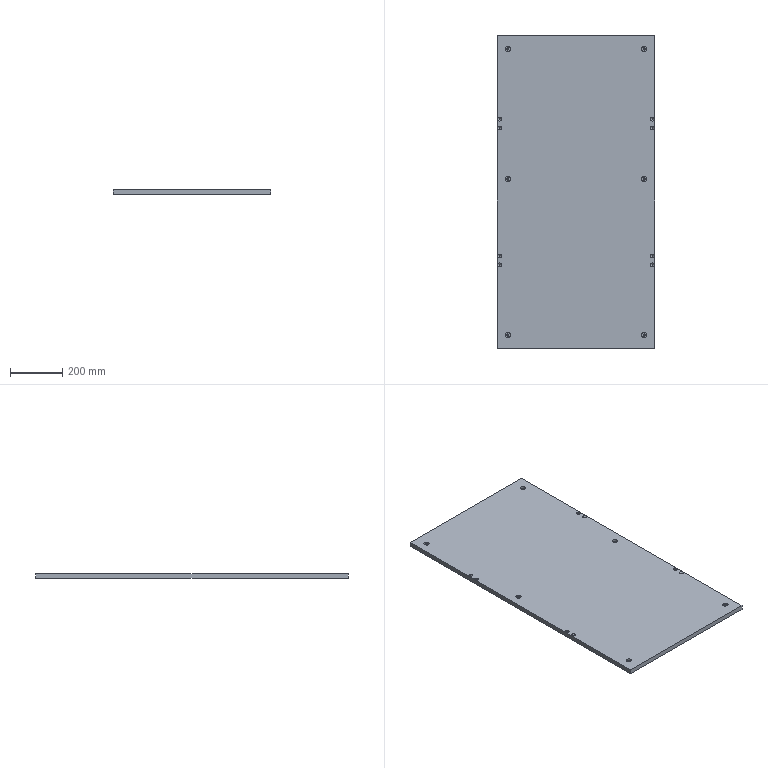Part | STEP file | DECAK 601 | 1 solid | 40 faces | box 605 x 1200 x 18 mm | volume 13042894 mm3 | cylinder 20 | plane 12 | cone 8 | commonest cylinder face diameters 6.5 x8 8.5 x6 20 x6